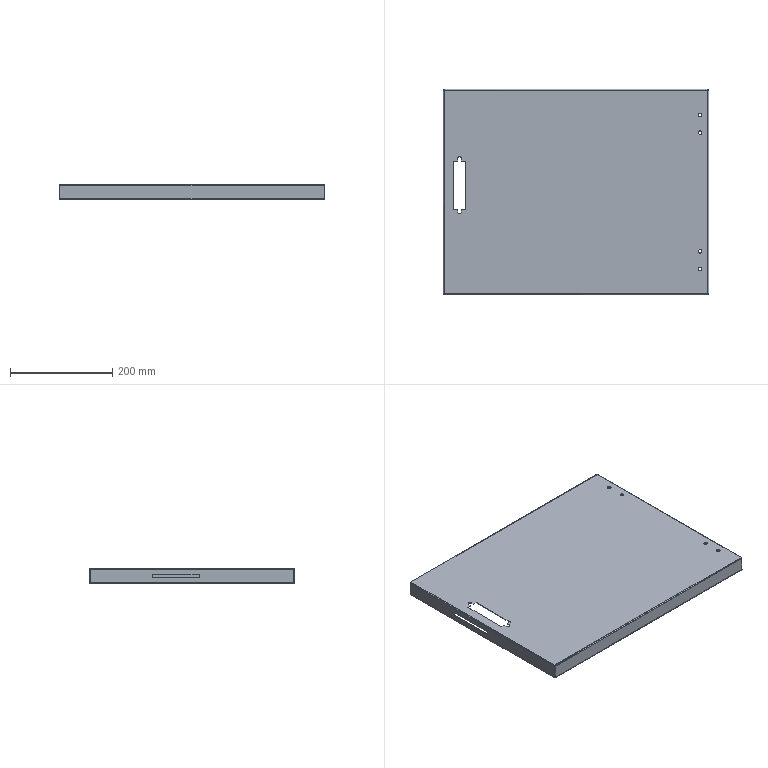Part | 1 solid | 95 faces | box 520 x 402 x 30 mm | volume 331167 mm3 | plane 50 | cylinder 29 | spline 16 | commonest cylinder face diameters 7 x13 1.473 x8 3.873 x8